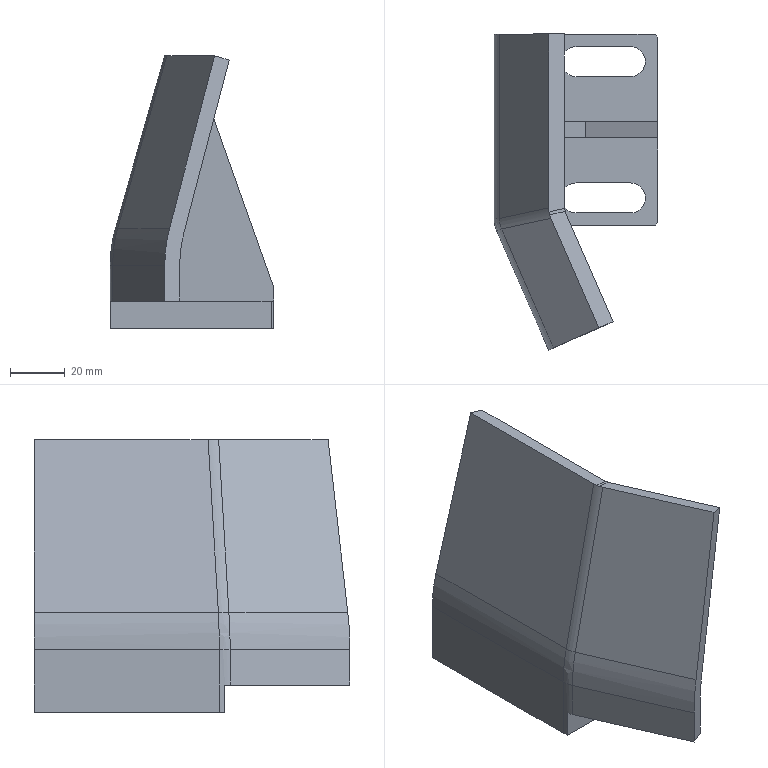Part | NX | features solid 2 | 1 solid | 44 faces | box 60 x 115.826 x 100 mm | volume 115790 mm3 | plane 28 | cylinder 14 | spline 2 | commonest cylinder face diameters 20 x5 11 x4 88 x3 100 x2
STEP:
#1=CARTESIAN_POINT('',(525.835,273.087,-27.003));
#2=VERTEX_POINT('',#1);
#3=CARTESIAN_POINT('',(545.,229.174,-27.003));
#4=VERTEX_POINT('',#3);
#5=CARTESIAN_POINT('',(525.,275.,-27.003));
#6=DIRECTION('',(0.4,-0.9165,0.));
#7=VECTOR('',#6,1000.);
#8=LINE('',#5,#7);
#9=EDGE_CURVE('',#2,#4,#8,.T.);
#10=ORIENTED_EDGE('',*,*,#9,.T.);
#11=CARTESIAN_POINT('',(546.763,229.944,-13.267));
#12=VERTEX_POINT('',#11);
#13=CARTESIAN_POINT('',(590.826,249.174,-27.003));
#14=DIRECTION('',(0.4,-0.9165,0.));
#15=DIRECTION('',(0.9165,0.4,0.));
#16=AXIS2_PLACEMENT_3D('',#13,#14,#15);
#17=CIRCLE('',#16,50.);
#18=EDGE_CURVE('',#12,#4,#17,.T.);
#19=ORIENTED_EDGE('',*,*,#18,.F.);
#20=CARTESIAN_POINT('',(527.727,273.562,-13.267));
#21=VERTEX_POINT('',#20);
#22=CARTESIAN_POINT('',(526.763,275.77,-13.267));
#23=DIRECTION('',(0.4,-0.9165,0.));
#24=VECTOR('',#23,1000.);
#25=LINE('',#22,#24);
#26=EDGE_CURVE('',#21,#12,#25,.T.);
#27=ORIENTED_EDGE('',*,*,#26,.F.);
#28=CARTESIAN_POINT('',(575.,285.436,-27.003));
#29=DIRECTION('',(-0.2436,0.9699,0.));
#30=DIRECTION('',(0.9699,0.2436,0.));
#31=AXIS2_PLACEMENT_3D('',#28,#29,#30);
#32=ELLIPSE('',#31,50.692,50.);
#33=EDGE_CURVE('',#2,#21,#32,.T.);
#34=ORIENTED_EDGE('',*,*,#33,.F.);
#35=EDGE_LOOP('',(#10,#19,#27,#34));
#36=FACE_BOUND('',#35,.T.);
#37=CARTESIAN_POINT('',(570.826,295.,-27.003));
#38=DIRECTION('',(0.4,-0.9165,0.));
#39=DIRECTION('',(-0.9165,-0.4,0.));
#40=AXIS2_PLACEMENT_3D('',#37,#38,#39);
#41=CYLINDRICAL_SURFACE('',#40,50.);
#42=ADVANCED_FACE('',(#36),#41,.T.);
#43=CARTESIAN_POINT('',(555.,279.5,-40.));
#44=VERTEX_POINT('',#43);
#45=CARTESIAN_POINT('',(575.,279.5,-40.));
#46=VERTEX_POINT('',#45);
#47=CARTESIAN_POINT('',(555.,279.5,-40.));
#48=DIRECTION('',(1.,0.,0.));
#49=VECTOR('',#48,1000.);
#50=LINE('',#47,#49);
#51=EDGE_CURVE('',#44,#46,#50,.T.);
#52=ORIENTED_EDGE('',*,*,#51,.F.);
#53=CARTESIAN_POINT('',(555.,290.5,-40.));
#54=VERTEX_POINT('',#53);
#55=CARTESIAN_POINT('',(555.,285.,-40.));
#56=DIRECTION('',(0.,0.,-1.));
#57=DIRECTION('',(1.,0.,0.));
#58=AXIS2_PLACEMENT_3D('',#55,#56,#57);
#59=CIRCLE('',#58,5.5);
#60=EDGE_CURVE('',#44,#54,#59,.T.);
#61=ORIENTED_EDGE('',*,*,#60,.T.);
#62=CARTESIAN_POINT('',(575.,290.5,-40.));
#63=VERTEX_POINT('',#62);
#64=CARTESIAN_POINT('',(575.,290.5,-40.));
#65=DIRECTION('',(-1.,0.,0.));
#66=VECTOR('',#65,1000.);
#67=LINE('',#64,#66);
#68=EDGE_CURVE('',#63,#54,#67,.T.);
#69=ORIENTED_EDGE('',*,*,#68,.F.);
#70=CARTESIAN_POINT('',(575.,285.,-40.));
#71=DIRECTION('',(0.,0.,-1.));
#72=DIRECTION('',(1.,0.,0.));
#73=AXIS2_PLACEMENT_3D('',#70,#71,#72);
#74=CIRCLE('',#73,5.5);
#75=EDGE_CURVE('',#63,#46,#74,.T.);
#76=ORIENTED_EDGE('',*,*,#75,.T.);
#77=EDGE_LOOP('',(#52,#61,#69,#76));
#78=FACE_BOUND('',#77,.T.);
#79=CARTESIAN_POINT('',(575.,340.5,-40.));
#80=VERTEX_POINT('',#79);
#81=CARTESIAN_POINT('',(555.,340.5,-40.));
#82=VERTEX_POINT('',#81);
#83=CARTESIAN_POINT('',(575.,340.5,-40.));
#84=DIRECTION('',(-1.,0.,0.));
#85=VECTOR('',#84,1000.);
#86=LINE('',#83,#85);
#87=EDGE_CURVE('',#80,#82,#86,.T.);
#88=ORIENTED_EDGE('',*,*,#87,.F.);
#89=CARTESIAN_POINT('',(575.,329.5,-40.));
#90=VERTEX_POINT('',#89);
#91=CARTESIAN_POINT('',(575.,335.,-40.));
#92=DIRECTION('',(0.,0.,-1.));
#93=DIRECTION('',(1.,0.,0.));
#94=AXIS2_PLACEMENT_3D('',#91,#92,#93);
#95=CIRCLE('',#94,5.5);
#96=EDGE_CURVE('',#80,#90,#95,.T.);
#97=ORIENTED_EDGE('',*,*,#96,.T.);
#98=CARTESIAN_POINT('',(555.,329.5,-40.));
#99=VERTEX_POINT('',#98);
#100=CARTESIAN_POINT('',(555.,329.5,-40.));
#101=DIRECTION('',(1.,0.,0.));
#102=VECTOR('',#101,1000.);
#103=LINE('',#100,#102);
#104=EDGE_CURVE('',#99,#90,#103,.T.);
#105=ORIENTED_EDGE('',*,*,#104,.F.);
#106=CARTESIAN_POINT('',(555.,335.,-40.));
#107=DIRECTION('',(0.,0.,-1.));
#108=DIRECTION('',(1.,0.,0.));
#109=AXIS2_PLACEMENT_3D('',#106,#107,#108);
#110=CIRCLE('',#109,5.5);
#111=EDGE_CURVE('',#99,#82,#110,.T.);
#112=ORIENTED_EDGE('',*,*,#111,.T.);
#113=EDGE_LOOP('',(#88,#97,#105,#112));
#114=FACE_BOUND('',#113,.T.);
#115=CARTESIAN_POINT('',(531.574,275.,-40.));
#116=VERTEX_POINT('',#115);
#117=CARTESIAN_POINT('',(584.,275.,-40.));
#118=VERTEX_POINT('',#117);
#119=CARTESIAN_POINT('',(525.,275.,-40.));
#120=DIRECTION('',(1.,0.,0.));
#121=VECTOR('',#120,1000.);
#122=LINE('',#119,#121);
#123=EDGE_CURVE('',#116,#118,#122,.T.);
#124=ORIENTED_EDGE('',*,*,#123,.T.);
#125=CARTESIAN_POINT('',(585.,276.,-40.));
#126=VERTEX_POINT('',#125);
#127=CARTESIAN_POINT('',(584.,275.,-40.));
#128=DIRECTION('',(0.7071,0.7071,0.));
#129=VECTOR('',#128,1000.);
#130=LINE('',#127,#129);
#131=EDGE_CURVE('',#118,#126,#130,.T.);
#132=ORIENTED_EDGE('',*,*,#131,.T.);
#133=CARTESIAN_POINT('',(585.,307.,-40.));
#134=VERTEX_POINT('',#133);
#135=CARTESIAN_POINT('',(585.,276.,-40.));
#136=DIRECTION('',(0.,1.,0.));
#137=VECTOR('',#136,1000.);
#138=LINE('',#135,#137);
#139=EDGE_CURVE('',#126,#134,#138,.T.);
#140=ORIENTED_EDGE('',*,*,#139,.T.);
#141=CARTESIAN_POINT('',(541.,307.,-40.));
#142=VERTEX_POINT('',#141);
#143=CARTESIAN_POINT('',(585.,307.,-40.));
#144=DIRECTION('',(-1.,0.,0.));
#145=VECTOR('',#144,1000.);
#146=LINE('',#143,#145);
#147=EDGE_CURVE('',#134,#142,#146,.T.);
#148=ORIENTED_EDGE('',*,*,#147,.T.);
#149=CARTESIAN_POINT('',(541.,313.,-40.));
#150=VERTEX_POINT('',#149);
#151=CARTESIAN_POINT('',(541.,307.,-40.));
#152=DIRECTION('',(0.,1.,0.));
#153=VECTOR('',#152,1000.);
#154=LINE('',#151,#153);
#155=EDGE_CURVE('',#142,#150,#154,.T.);
#156=ORIENTED_EDGE('',*,*,#155,.T.);
#157=CARTESIAN_POINT('',(585.,313.,-40.));
#158=VERTEX_POINT('',#157);
#159=CARTESIAN_POINT('',(585.,313.,-40.));
#160=DIRECTION('',(-1.,0.,0.));
#161=VECTOR('',#160,1000.);
#162=LINE('',#159,#161);
#163=EDGE_CURVE('',#158,#150,#162,.T.);
#164=ORIENTED_EDGE('',*,*,#163,.F.);
#165=CARTESIAN_POINT('',(585.,344.,-40.));
#166=VERTEX_POINT('',#165);
#167=CARTESIAN_POINT('',(585.,276.,-40.));
#168=DIRECTION('',(0.,1.,0.));
#169=VECTOR('',#168,1000.);
#170=LINE('',#167,#169);
#171=EDGE_CURVE('',#158,#166,#170,.T.);
#172=ORIENTED_EDGE('',*,*,#171,.T.);
#173=CARTESIAN_POINT('',(584.,345.,-40.));
#174=VERTEX_POINT('',#173);
#175=CARTESIAN_POINT('',(585.,344.,-40.));
#176=DIRECTION('',(-0.7071,0.7071,0.));
#177=VECTOR('',#176,1000.);
#178=LINE('',#175,#177);
#179=EDGE_CURVE('',#166,#174,#178,.T.);
#180=ORIENTED_EDGE('',*,*,#179,.T.);
#181=CARTESIAN_POINT('',(531.,345.,-40.));
#182=VERTEX_POINT('',#181);
#183=CARTESIAN_POINT('',(584.,345.,-40.));
#184=DIRECTION('',(-1.,0.,0.));
#185=VECTOR('',#184,1000.);
#186=LINE('',#183,#185);
#187=EDGE_CURVE('',#174,#182,#186,.T.);
#188=ORIENTED_EDGE('',*,*,#187,.T.);
#189=CARTESIAN_POINT('',(531.,278.339,-40.));
#190=VERTEX_POINT('',#189);
#191=CARTESIAN_POINT('',(531.,275.,-40.));
#192=DIRECTION('',(0.,1.,0.));
#193=VECTOR('',#192,1000.);
#194=LINE('',#191,#193);
#195=EDGE_CURVE('',#190,#182,#194,.T.);
#196=ORIENTED_EDGE('',*,*,#195,.F.);
#197=CARTESIAN_POINT('',(541.,278.339,-40.));
#198=DIRECTION('',(0.,0.,1.));
#199=DIRECTION('',(-1.,0.,0.));
#200=AXIS2_PLACEMENT_3D('',#197,#198,#199);
#201=CIRCLE('',#200,10.);
#202=EDGE_CURVE('',#116,#190,#201,.F.);
#203=ORIENTED_EDGE('',*,*,#202,.F.);
#204=EDGE_LOOP('',(#124,#132,#140,#148,#156,#164,#172,#180,#188,#196,#203));
#205=FACE_BOUND('',#204,.T.);
#206=CARTESIAN_POINT('',(525.,275.,-40.));
#207=DIRECTION('',(0.,0.,-1.));
#208=DIRECTION('',(-1.,0.,0.));
#209=AXIS2_PLACEMENT_3D('',#206,#207,#208);
#210=PLANE('',#209);
#211=ADVANCED_FACE('',(#78,#114,#205),#210,.F.);
#212=CARTESIAN_POINT('',(525.,277.087,-27.003));
#213=VERTEX_POINT('',#212);
#214=CARTESIAN_POINT('',(525.,345.,-27.003));
#215=VERTEX_POINT('',#214);
#216=CARTESIAN_POINT('',(525.,275.,-27.003));
#217=DIRECTION('',(0.,1.,0.));
#218=VECTOR('',#217,1000.);
#219=LINE('',#216,#218);
#220=EDGE_CURVE('',#213,#215,#219,.T.);
#221=ORIENTED_EDGE('',*,*,#220,.T.);
#222=CARTESIAN_POINT('',(525.,345.,-50.));
#223=VERTEX_POINT('',#222);
#224=CARTESIAN_POINT('',(525.,345.,-40.));
#225=DIRECTION('',(0.,0.,-1.));
#226=VECTOR('',#225,1000.);
#227=LINE('',#224,#226);
#228=EDGE_CURVE('',#215,#223,#227,.T.);
#229=ORIENTED_EDGE('',*,*,#228,.T.);
#230=CARTESIAN_POINT('',(525.,277.087,-50.));
#231=VERTEX_POINT('',#230);
#232=CARTESIAN_POINT('',(525.,345.,-50.));
#233=DIRECTION('',(0.,-1.,0.));
#234=VECTOR('',#233,1000.);
#235=LINE('',#232,#234);
#236=EDGE_CURVE('',#223,#231,#235,.T.);
#237=ORIENTED_EDGE('',*,*,#236,.T.);
#238=CARTESIAN_POINT('',(525.,277.087,-40.));
#239=DIRECTION('',(0.,0.,-1.));
#240=VECTOR('',#239,1000.);
#241=LINE('',#238,#240);
#242=EDGE_CURVE('',#213,#231,#241,.T.);
#243=ORIENTED_EDGE('',*,*,#242,.F.);
#244=EDGE_LOOP('',(#221,#229,#237,#243));
#245=FACE_BOUND('',#244,.T.);
#246=CARTESIAN_POINT('',(525.,345.,-40.));
#247=DIRECTION('',(-1.,0.,0.));
#248=DIRECTION('',(0.,0.,1.));
#249=AXIS2_PLACEMENT_3D('',#246,#247,#248);
#250=PLANE('',#249);
#251=ADVANCED_FACE('',(#245),#250,.T.);
#252=CARTESIAN_POINT('',(525.22,275.,-50.));
#253=VERTEX_POINT('',#252);
#254=CARTESIAN_POINT('',(584.,275.,-50.));
#255=VERTEX_POINT('',#254);
#256=CARTESIAN_POINT('',(525.,275.,-50.));
#257=DIRECTION('',(1.,0.,0.));
#258=VECTOR('',#257,1000.);
#259=LINE('',#256,#258);
#260=EDGE_CURVE('',#253,#255,#259,.T.);
#261=ORIENTED_EDGE('',*,*,#260,.T.);
#262=CARTESIAN_POINT('',(584.,275.,-40.));
#263=DIRECTION('',(0.,0.,-1.));
#264=VECTOR('',#263,1000.);
#265=LINE('',#262,#264);
#266=EDGE_CURVE('',#118,#255,#265,.T.);
#267=ORIENTED_EDGE('',*,*,#266,.F.);
#268=ORIENTED_EDGE('',*,*,#123,.F.);
#269=CARTESIAN_POINT('',(525.22,275.,-40.));
#270=VERTEX_POINT('',#269);
#271=CARTESIAN_POINT('',(525.,275.,-40.));
#272=DIRECTION('',(1.,0.,0.));
#273=VECTOR('',#272,1000.);
#274=LINE('',#271,#273);
#275=EDGE_CURVE('',#270,#116,#274,.T.);
#276=ORIENTED_EDGE('',*,*,#275,.F.);
#277=CARTESIAN_POINT('',(525.22,275.,-50.));
#278=DIRECTION('',(0.,0.,-1.));
#279=VECTOR('',#278,1000.);
#280=LINE('',#277,#279);
#281=EDGE_CURVE('',#253,#270,#280,.F.);
#282=ORIENTED_EDGE('',*,*,#281,.F.);
#283=EDGE_LOOP('',(#261,#267,#268,#276,#282));
#284=FACE_BOUND('',#283,.T.);
#285=CARTESIAN_POINT('',(525.,275.,-40.));
#286=DIRECTION('',(0.,-1.,0.));
#287=DIRECTION('',(0.,0.,1.));
#288=AXIS2_PLACEMENT_3D('',#285,#286,#287);
#289=PLANE('',#288);
#290=ADVANCED_FACE('',(#284),#289,.T.);
#291=CARTESIAN_POINT('',(585.,276.,-50.));
#292=VERTEX_POINT('',#291);
#293=CARTESIAN_POINT('',(584.,275.,-50.));
#294=DIRECTION('',(0.7071,0.7071,0.));
#295=VECTOR('',#294,1000.);
#296=LINE('',#293,#295);
#297=EDGE_CURVE('',#255,#292,#296,.T.);
#298=ORIENTED_EDGE('',*,*,#297,.T.);
#299=CARTESIAN_POINT('',(585.,276.,-40.));
#300=DIRECTION('',(0.,0.,-1.));
#301=VECTOR('',#300,1000.);
#302=LINE('',#299,#301);
#303=EDGE_CURVE('',#126,#292,#302,.T.);
#304=ORIENTED_EDGE('',*,*,#303,.F.);
#305=ORIENTED_EDGE('',*,*,#131,.F.);
#306=ORIENTED_EDGE('',*,*,#266,.T.);
#307=EDGE_LOOP('',(#298,#304,#305,#306));
#308=FACE_BOUND('',#307,.T.);
#309=CARTESIAN_POINT('',(584.,275.,-40.));
#310=DIRECTION('',(0.7071,-0.7071,0.));
#311=DIRECTION('',(-0.7071,-0.7071,0.));
#312=AXIS2_PLACEMENT_3D('',#309,#310,#311);
#313=PLANE('',#312);
#314=ADVANCED_FACE('',(#308),#313,.T.);
#315=CARTESIAN_POINT('',(585.,344.,-50.));
#316=VERTEX_POINT('',#315);
#317=CARTESIAN_POINT('',(585.,276.,-50.));
#318=DIRECTION('',(0.,1.,0.));
#319=VECTOR('',#318,1000.);
#320=LINE('',#317,#319);
#321=EDGE_CURVE('',#292,#316,#320,.T.);
#322=ORIENTED_EDGE('',*,*,#321,.T.);
#323=CARTESIAN_POINT('',(585.,344.,-40.));
#324=DIRECTION('',(0.,0.,-1.));
#325=VECTOR('',#324,1000.);
#326=LINE('',#323,#325);
#327=EDGE_CURVE('',#166,#316,#326,.T.);
#328=ORIENTED_EDGE('',*,*,#327,.F.);
#329=ORIENTED_EDGE('',*,*,#171,.F.);
#330=CARTESIAN_POINT('',(585.,313.,-35.));
#331=VERTEX_POINT('',#330);
#332=CARTESIAN_POINT('',(585.,313.,-35.));
#333=DIRECTION('',(0.,0.,-1.));
#334=VECTOR('',#333,1000.);
#335=LINE('',#332,#334);
#336=EDGE_CURVE('',#331,#158,#335,.T.);
#337=ORIENTED_EDGE('',*,*,#336,.F.);
#338=CARTESIAN_POINT('',(585.,307.,-35.));
#339=VERTEX_POINT('',#338);
#340=CARTESIAN_POINT('',(585.,307.,-35.));
#341=DIRECTION('',(0.,1.,0.));
#342=VECTOR('',#341,1000.);
#343=LINE('',#340,#342);
#344=EDGE_CURVE('',#339,#331,#343,.T.);
#345=ORIENTED_EDGE('',*,*,#344,.F.);
#346=CARTESIAN_POINT('',(585.,307.,-35.));
#347=DIRECTION('',(0.,0.,-1.));
#348=VECTOR('',#347,1000.);
#349=LINE('',#346,#348);
#350=EDGE_CURVE('',#339,#134,#349,.T.);
#351=ORIENTED_EDGE('',*,*,#350,.T.);
#352=ORIENTED_EDGE('',*,*,#139,.F.);
#353=ORIENTED_EDGE('',*,*,#303,.T.);
#354=EDGE_LOOP('',(#322,#328,#329,#337,#345,#351,#352,#353));
#355=FACE_BOUND('',#354,.T.);
#356=CARTESIAN_POINT('',(585.,276.,-40.));
#357=DIRECTION('',(1.,0.,0.));
#358=DIRECTION('',(0.,-1.,0.));
#359=AXIS2_PLACEMENT_3D('',#356,#357,#358);
#360=PLANE('',#359);
#361=ADVANCED_FACE('',(#355),#360,.T.);
#362=CARTESIAN_POINT('',(584.,345.,-50.));
#363=VERTEX_POINT('',#362);
#364=CARTESIAN_POINT('',(585.,344.,-50.));
#365=DIRECTION('',(-0.7071,0.7071,0.));
#366=VECTOR('',#365,1000.);
#367=LINE('',#364,#366);
#368=EDGE_CURVE('',#316,#363,#367,.T.);
#369=ORIENTED_EDGE('',*,*,#368,.T.);
#370=CARTESIAN_POINT('',(584.,345.,-40.));
#371=DIRECTION('',(0.,0.,-1.));
#372=VECTOR('',#371,1000.);
#373=LINE('',#370,#372);
#374=EDGE_CURVE('',#174,#363,#373,.T.);
#375=ORIENTED_EDGE('',*,*,#374,.F.);
#376=ORIENTED_EDGE('',*,*,#179,.F.);
#377=ORIENTED_EDGE('',*,*,#327,.T.);
#378=EDGE_LOOP('',(#369,#375,#376,#377));
#379=FACE_BOUND('',#378,.T.);
#380=CARTESIAN_POINT('',(585.,344.,-40.));
#381=DIRECTION('',(0.7071,0.7071,0.));
#382=DIRECTION('',(0.7071,-0.7071,0.));
#383=AXIS2_PLACEMENT_3D('',#380,#381,#382);
#384=PLANE('',#383);
#385=ADVANCED_FACE('',(#379),#384,.T.);
#386=CARTESIAN_POINT('',(555.,279.5,-50.));
#387=VERTEX_POINT('',#386);
#388=CARTESIAN_POINT('',(575.,279.5,-50.));
#389=VERTEX_POINT('',#388);
#390=CARTESIAN_POINT('',(555.,279.5,-50.));
#391=DIRECTION('',(1.,0.,0.));
#392=VECTOR('',#391,1000.);
#393=LINE('',#390,#392);
#394=EDGE_CURVE('',#387,#389,#393,.T.);
#395=ORIENTED_EDGE('',*,*,#394,.F.);
#396=CARTESIAN_POINT('',(555.,279.5,-40.));
#397=DIRECTION('',(0.,0.,-1.));
#398=VECTOR('',#397,1000.);
#399=LINE('',#396,#398);
#400=EDGE_CURVE('',#44,#387,#399,.T.);
#401=ORIENTED_EDGE('',*,*,#400,.F.);
#402=ORIENTED_EDGE('',*,*,#51,.T.);
#403=CARTESIAN_POINT('',(575.,279.5,-40.));
#404=DIRECTION('',(0.,0.,-1.));
#405=VECTOR('',#404,1000.);
#406=LINE('',#403,#405);
#407=EDGE_CURVE('',#46,#389,#406,.T.);
#408=ORIENTED_EDGE('',*,*,#407,.T.);
#409=EDGE_LOOP('',(#395,#401,#402,#408));
#410=FACE_BOUND('',#409,.T.);
#411=CARTESIAN_POINT('',(555.,279.5,-40.));
#412=DIRECTION('',(0.,-1.,0.));
#413=DIRECTION('',(0.,0.,1.));
#414=AXIS2_PLACEMENT_3D('',#411,#412,#413);
#415=PLANE('',#414);
#416=ADVANCED_FACE('',(#410),#415,.F.);
#417=CARTESIAN_POINT('',(555.,290.5,-50.));
#418=VERTEX_POINT('',#417);
#419=CARTESIAN_POINT('',(555.,285.,-50.));
#420=DIRECTION('',(0.,0.,-1.));
#421=DIRECTION('',(1.,0.,0.));
#422=AXIS2_PLACEMENT_3D('',#419,#420,#421);
#423=CIRCLE('',#422,5.5);
#424=EDGE_CURVE('',#387,#418,#423,.T.);
#425=ORIENTED_EDGE('',*,*,#424,.T.);
#426=CARTESIAN_POINT('',(555.,290.5,-40.));
#427=DIRECTION('',(0.,0.,-1.));
#428=VECTOR('',#427,1000.);
#429=LINE('',#426,#428);
#430=EDGE_CURVE('',#54,#418,#429,.T.);
#431=ORIENTED_EDGE('',*,*,#430,.F.);
#432=ORIENTED_EDGE('',*,*,#60,.F.);
#433=ORIENTED_EDGE('',*,*,#400,.T.);
#434=EDGE_LOOP('',(#425,#431,#432,#433));
#435=FACE_BOUND('',#434,.T.);
#436=CARTESIAN_POINT('',(555.,285.,-40.));
#437=DIRECTION('',(0.,0.,-1.));
#438=DIRECTION('',(-1.,0.,0.));
#439=AXIS2_PLACEMENT_3D('',#436,#437,#438);
#440=CYLINDRICAL_SURFACE('',#439,5.5);
#441=ADVANCED_FACE('',(#435),#440,.F.);
#442=CARTESIAN_POINT('',(575.,290.5,-50.));
#443=VERTEX_POINT('',#442);
#444=CARTESIAN_POINT('',(575.,290.5,-50.));
#445=DIRECTION('',(-1.,0.,0.));
#446=VECTOR('',#445,1000.);
#447=LINE('',#444,#446);
#448=EDGE_CURVE('',#443,#418,#447,.T.);
#449=ORIENTED_EDGE('',*,*,#448,.F.);
#450=CARTESIAN_POINT('',(575.,290.5,-40.));
#451=DIRECTION('',(0.,0.,-1.));
#452=VECTOR('',#451,1000.);
#453=LINE('',#450,#452);
#454=EDGE_CURVE('',#63,#443,#453,.T.);
#455=ORIENTED_EDGE('',*,*,#454,.F.);
#456=ORIENTED_EDGE('',*,*,#68,.T.);
#457=ORIENTED_EDGE('',*,*,#430,.T.);
#458=EDGE_LOOP('',(#449,#455,#456,#457));
#459=FACE_BOUND('',#458,.T.);
#460=CARTESIAN_POINT('',(575.,290.5,-40.));
#461=DIRECTION('',(0.,1.,0.));
#462=DIRECTION('',(0.,0.,-1.));
#463=AXIS2_PLACEMENT_3D('',#460,#461,#462);
#464=PLANE('',#463);
#465=ADVANCED_FACE('',(#459),#464,.F.);
#466=CARTESIAN_POINT('',(575.,340.5,-50.));
#467=VERTEX_POINT('',#466);
#468=CARTESIAN_POINT('',(555.,340.5,-50.));
#469=VERTEX_POINT('',#468);
#470=CARTESIAN_POINT('',(575.,340.5,-50.));
#471=DIRECTION('',(-1.,0.,0.));
#472=VECTOR('',#471,1000.);
#473=LINE('',#470,#472);
#474=EDGE_CURVE('',#467,#469,#473,.T.);
#475=ORIENTED_EDGE('',*,*,#474,.F.);
#476=CARTESIAN_POINT('',(575.,340.5,-40.));
#477=DIRECTION('',(0.,0.,-1.));
#478=VECTOR('',#477,1000.);
#479=LINE('',#476,#478);
#480=EDGE_CURVE('',#80,#467,#479,.T.);
#481=ORIENTED_EDGE('',*,*,#480,.F.);
#482=ORIENTED_EDGE('',*,*,#87,.T.);
#483=CARTESIAN_POINT('',(555.,340.5,-40.));
#484=DIRECTION('',(0.,0.,-1.));
#485=VECTOR('',#484,1000.);
#486=LINE('',#483,#485);
#487=EDGE_CURVE('',#82,#469,#486,.T.);
#488=ORIENTED_EDGE('',*,*,#487,.T.);
#489=EDGE_LOOP('',(#475,#481,#482,#488));
#490=FACE_BOUND('',#489,.T.);
#491=CARTESIAN_POINT('',(575.,340.5,-40.));
#492=DIRECTION('',(0.,1.,0.));
#493=DIRECTION('',(0.,0.,-1.));
#494=AXIS2_PLACEMENT_3D('',#491,#492,#493);
#495=PLANE('',#494);
#496=ADVANCED_FACE('',(#490),#495,.F.);
#497=CARTESIAN_POINT('',(575.,329.5,-50.));
#498=VERTEX_POINT('',#497);
#499=CARTESIAN_POINT('',(575.,335.,-50.));
#500=DIRECTION('',(0.,0.,-1.));
#501=DIRECTION('',(1.,0.,0.));
#502=AXIS2_PLACEMENT_3D('',#499,#500,#501);
#503=CIRCLE('',#502,5.5);
#504=EDGE_CURVE('',#467,#498,#503,.T.);
#505=ORIENTED_EDGE('',*,*,#504,.T.);
#506=CARTESIAN_POINT('',(575.,329.5,-40.));
#507=DIRECTION('',(0.,0.,-1.));
#508=VECTOR('',#507,1000.);
#509=LINE('',#506,#508);
#510=EDGE_CURVE('',#90,#498,#509,.T.);
#511=ORIENTED_EDGE('',*,*,#510,.F.);
#512=ORIENTED_EDGE('',*,*,#96,.F.);
#513=ORIENTED_EDGE('',*,*,#480,.T.);
#514=EDGE_LOOP('',(#505,#511,#512,#513));
#515=FACE_BOUND('',#514,.T.);
#516=CARTESIAN_POINT('',(575.,335.,-40.));
#517=DIRECTION('',(0.,0.,-1.));
#518=DIRECTION('',(-1.,0.,0.));
#519=AXIS2_PLACEMENT_3D('',#516,#517,#518);
#520=CYLINDRICAL_SURFACE('',#519,5.5);
#521=ADVANCED_FACE('',(#515),#520,.F.);
#522=CARTESIAN_POINT('',(555.,329.5,-50.));
#523=VERTEX_POINT('',#522);
#524=CARTESIAN_POINT('',(555.,329.5,-50.));
#525=DIRECTION('',(1.,0.,0.));
#526=VECTOR('',#525,1000.);
#527=LINE('',#524,#526);
#528=EDGE_CURVE('',#523,#498,#527,.T.);
#529=ORIENTED_EDGE('',*,*,#528,.F.);
#530=CARTESIAN_POINT('',(555.,329.5,-40.));
#531=DIRECTION('',(0.,0.,-1.));
#532=VECTOR('',#531,1000.);
#533=LINE('',#530,#532);
#534=EDGE_CURVE('',#99,#523,#533,.T.);
#535=ORIENTED_EDGE('',*,*,#534,.F.);
#536=ORIENTED_EDGE('',*,*,#104,.T.);
#537=ORIENTED_EDGE('',*,*,#510,.T.);
#538=EDGE_LOOP('',(#529,#535,#536,#537));
#539=FACE_BOUND('',#538,.T.);
#540=CARTESIAN_POINT('',(555.,329.5,-40.));
#541=DIRECTION('',(0.,-1.,0.));
#542=DIRECTION('',(0.,0.,1.));
#543=AXIS2_PLACEMENT_3D('',#540,#541,#542);
#544=PLANE('',#543);
#545=ADVANCED_FACE('',(#539),#544,.F.);
#546=CARTESIAN_POINT('',(575.,285.,-50.));
#547=DIRECTION('',(0.,0.,-1.));
#548=DIRECTION('',(1.,0.,0.));
#549=AXIS2_PLACEMENT_3D('',#546,#547,#548);
#550=CIRCLE('',#549,5.5);
#551=EDGE_CURVE('',#443,#389,#550,.T.);
#552=ORIENTED_EDGE('',*,*,#551,.T.);
#553=ORIENTED_EDGE('',*,*,#407,.F.);
#554=ORIENTED_EDGE('',*,*,#75,.F.);
#555=ORIENTED_EDGE('',*,*,#454,.T.);
#556=EDGE_LOOP('',(#552,#553,#554,#555));
#557=FACE_BOUND('',#556,.T.);
#558=CARTESIAN_POINT('',(575.,285.,-40.));
#559=DIRECTION('',(0.,0.,-1.));
#560=DIRECTION('',(-1.,0.,0.));
#561=AXIS2_PLACEMENT_3D('',#558,#559,#560);
#562=CYLINDRICAL_SURFACE('',#561,5.5);
#563=ADVANCED_FACE('',(#557),#562,.F.);
#564=CARTESIAN_POINT('',(555.,335.,-50.));
#565=DIRECTION('',(0.,0.,-1.));
#566=DIRECTION('',(1.,0.,0.));
#567=AXIS2_PLACEMENT_3D('',#564,#565,#566);
#568=CIRCLE('',#567,5.5);
#569=EDGE_CURVE('',#523,#469,#568,.T.);
#570=ORIENTED_EDGE('',*,*,#569,.T.);
#571=ORIENTED_EDGE('',*,*,#487,.F.);
#572=ORIENTED_EDGE('',*,*,#111,.F.);
#573=ORIENTED_EDGE('',*,*,#534,.T.);
#574=EDGE_LOOP('',(#570,#571,#572,#573));
#575=FACE_BOUND('',#574,.T.);
#576=CARTESIAN_POINT('',(555.,335.,-40.));
#577=DIRECTION('',(0.,0.,-1.));
#578=DIRECTION('',(-1.,0.,0.));
#579=AXIS2_PLACEMENT_3D('',#576,#577,#578);
#580=CYLINDRICAL_SURFACE('',#579,5.5);
#581=ADVANCED_FACE('',(#575),#580,.F.);
#582=CARTESIAN_POINT('',(584.,345.,-50.));
#583=DIRECTION('',(-1.,0.,0.));
#584=VECTOR('',#583,1000.);
#585=LINE('',#582,#584);
#586=EDGE_CURVE('',#363,#223,#585,.T.);
#587=ORIENTED_EDGE('',*,*,#586,.T.);
#588=ORIENTED_EDGE('',*,*,#228,.F.);
#589=CARTESIAN_POINT('',(526.924,345.,-13.267));
#590=VERTEX_POINT('',#589);
#591=CARTESIAN_POINT('',(575.,345.,-27.003));
#592=DIRECTION('',(0.,-1.,0.));
#593=DIRECTION('',(1.,0.,0.));
#594=AXIS2_PLACEMENT_3D('',#591,#592,#593);
#595=CIRCLE('',#594,50.);
#596=EDGE_CURVE('',#590,#215,#595,.T.);
#597=ORIENTED_EDGE('',*,*,#596,.F.);
#598=CARTESIAN_POINT('',(545.,345.,50.));
#599=VERTEX_POINT('',#598);
#600=CARTESIAN_POINT('',(526.924,345.,-13.267));
#601=DIRECTION('',(0.2747,0.,0.9615));
#602=VECTOR('',#601,1000.);
#603=LINE('',#600,#602);
#604=EDGE_CURVE('',#590,#599,#603,.T.);
#605=ORIENTED_EDGE('',*,*,#604,.T.);
#606=CARTESIAN_POINT('',(550.769,345.,48.352));
#607=VERTEX_POINT('',#606);
#608=CARTESIAN_POINT('',(545.,345.,50.));
#609=DIRECTION('',(0.9615,0.,-0.2747));
#610=VECTOR('',#609,1000.);
#611=LINE('',#608,#610);
#612=EDGE_CURVE('',#599,#607,#611,.T.);
#613=ORIENTED_EDGE('',*,*,#612,.T.);
#614=CARTESIAN_POINT('',(532.693,345.,-14.915));
#615=VERTEX_POINT('',#614);
#616=CARTESIAN_POINT('',(532.693,345.,-14.915));
#617=DIRECTION('',(0.2747,0.,0.9615));
#618=VECTOR('',#617,1000.);
#619=LINE('',#616,#618);
#620=EDGE_CURVE('',#615,#607,#619,.T.);
#621=ORIENTED_EDGE('',*,*,#620,.F.);
#622=CARTESIAN_POINT('',(531.,345.,-27.003));
#623=VERTEX_POINT('',#622);
#624=CARTESIAN_POINT('',(575.,345.,-27.003));
#625=DIRECTION('',(0.,-1.,0.));
#626=DIRECTION('',(1.,0.,0.));
#627=AXIS2_PLACEMENT_3D('',#624,#625,#626);
#628=CIRCLE('',#627,44.);
#629=EDGE_CURVE('',#615,#623,#628,.T.);
#630=ORIENTED_EDGE('',*,*,#629,.T.);
#631=CARTESIAN_POINT('',(531.,345.,-27.003));
#632=DIRECTION('',(0.,0.,-1.));
#633=VECTOR('',#632,1000.);
#634=LINE('',#631,#633);
#635=EDGE_CURVE('',#623,#182,#634,.T.);
#636=ORIENTED_EDGE('',*,*,#635,.T.);
#637=ORIENTED_EDGE('',*,*,#187,.F.);
#638=ORIENTED_EDGE('',*,*,#374,.T.);
#639=EDGE_LOOP('',(#587,#588,#597,#605,#613,#621,#630,#636,#637,#638));
#640=FACE_BOUND('',#639,.T.);
#641=CARTESIAN_POINT('',(584.,345.,-40.));
#642=DIRECTION('',(0.,1.,0.));
#643=DIRECTION('',(1.,0.,0.));
#644=AXIS2_PLACEMENT_3D('',#641,#642,#643);
#645=PLANE('',#644);
#646=ADVANCED_FACE('',(#640),#645,.T.);
#647=ORIENTED_EDGE('',*,*,#474,.T.);
#648=ORIENTED_EDGE('',*,*,#569,.F.);
#649=ORIENTED_EDGE('',*,*,#528,.T.);
#650=ORIENTED_EDGE('',*,*,#504,.F.);
#651=EDGE_LOOP('',(#647,#648,#649,#650));
#652=FACE_BOUND('',#651,.T.);
#653=ORIENTED_EDGE('',*,*,#394,.T.);
#654=ORIENTED_EDGE('',*,*,#551,.F.);
#655=ORIENTED_EDGE('',*,*,#448,.T.);
#656=ORIENTED_EDGE('',*,*,#424,.F.);
#657=EDGE_LOOP('',(#653,#654,#655,#656));
#658=FACE_BOUND('',#657,.T.);
#659=ORIENTED_EDGE('',*,*,#236,.F.);
#660=ORIENTED_EDGE('',*,*,#586,.F.);
#661=ORIENTED_EDGE('',*,*,#368,.F.);
#662=ORIENTED_EDGE('',*,*,#321,.F.);
#663=ORIENTED_EDGE('',*,*,#297,.F.);
#664=ORIENTED_EDGE('',*,*,#260,.F.);
#665=CARTESIAN_POINT('',(535.,277.087,-50.));
#666=DIRECTION('',(0.,0.,1.));
#667=DIRECTION('',(-1.,0.,0.));
#668=AXIS2_PLACEMENT_3D('',#665,#666,#667);
#669=CIRCLE('',#668,10.);
#670=EDGE_CURVE('',#231,#253,#669,.T.);
#671=ORIENTED_EDGE('',*,*,#670,.F.);
#672=EDGE_LOOP('',(#659,#660,#661,#662,#663,#664,#671));
#673=FACE_BOUND('',#672,.T.);
#674=CARTESIAN_POINT('',(525.,275.,-50.));
#675=DIRECTION('',(0.,0.,-1.));
#676=DIRECTION('',(-1.,0.,0.));
#677=AXIS2_PLACEMENT_3D('',#674,#675,#676);
#678=PLANE('',#677);
#679=ADVANCED_FACE('',(#652,#658,#673),#678,.T.);
#680=CARTESIAN_POINT('',(548.383,313.,40.));
#681=VERTEX_POINT('',#680);
#682=CARTESIAN_POINT('',(558.383,313.,40.));
#683=VERTEX_POINT('',#682);
#684=CARTESIAN_POINT('',(548.383,313.,40.));
#685=DIRECTION('',(1.,0.,0.));
#686=VECTOR('',#685,1000.);
#687=LINE('',#684,#686);
#688=EDGE_CURVE('',#681,#683,#687,.T.);
#689=ORIENTED_EDGE('',*,*,#688,.F.);
#690=CARTESIAN_POINT('',(548.383,307.,40.));
#691=VERTEX_POINT('',#690);
#692=CARTESIAN_POINT('',(548.383,307.,40.));
#693=DIRECTION('',(0.,1.,0.));
#694=VECTOR('',#693,1000.);
#695=LINE('',#692,#694);
#696=EDGE_CURVE('',#691,#681,#695,.T.);
#697=ORIENTED_EDGE('',*,*,#696,.F.);
#698=CARTESIAN_POINT('',(558.383,307.,40.));
#699=VERTEX_POINT('',#698);
#700=CARTESIAN_POINT('',(548.383,307.,40.));
#701=DIRECTION('',(1.,0.,0.));
#702=VECTOR('',#701,1000.);
#703=LINE('',#700,#702);
#704=EDGE_CURVE('',#691,#699,#703,.T.);
#705=ORIENTED_EDGE('',*,*,#704,.T.);
#706=CARTESIAN_POINT('',(558.383,307.,40.));
#707=DIRECTION('',(0.,1.,0.));
#708=VECTOR('',#707,1000.);
#709=LINE('',#706,#708);
#710=EDGE_CURVE('',#699,#683,#709,.T.);
#711=ORIENTED_EDGE('',*,*,#710,.T.);
#712=EDGE_LOOP('',(#689,#697,#705,#711));
#713=FACE_BOUND('',#712,.T.);
#714=CARTESIAN_POINT('',(548.383,307.,40.));
#715=DIRECTION('',(0.,0.,-1.));
#716=DIRECTION('',(-1.,0.,0.));
#717=AXIS2_PLACEMENT_3D('',#714,#715,#716);
#718=PLANE('',#717);
#719=ADVANCED_FACE('',(#713),#718,.F.);
#720=CARTESIAN_POINT('',(558.383,313.,40.));
#721=DIRECTION('',(0.3345,0.,-0.9424));
#722=VECTOR('',#721,1000.);
#723=LINE('',#720,#722);
#724=EDGE_CURVE('',#683,#331,#723,.T.);
#725=ORIENTED_EDGE('',*,*,#724,.F.);
#726=ORIENTED_EDGE('',*,*,#710,.F.);
#727=CARTESIAN_POINT('',(558.383,307.,40.));
#728=DIRECTION('',(0.3345,0.,-0.9424));
#729=VECTOR('',#728,1000.);
#730=LINE('',#727,#729);
#731=EDGE_CURVE('',#699,#339,#730,.T.);
#732=ORIENTED_EDGE('',*,*,#731,.T.);
#733=ORIENTED_EDGE('',*,*,#344,.T.);
#734=EDGE_LOOP('',(#725,#726,#732,#733));
#735=FACE_BOUND('',#734,.T.);
#736=CARTESIAN_POINT('',(558.383,307.,40.));
#737=DIRECTION('',(-0.9424,0.,-0.3345));
#738=DIRECTION('',(-0.3345,0.,0.9424));
#739=AXIS2_PLACEMENT_3D('',#736,#737,#738);
#740=PLANE('',#739);
#741=ADVANCED_FACE('',(#735),#740,.F.);
#742=ORIENTED_EDGE('',*,*,#147,.F.);
#743=ORIENTED_EDGE('',*,*,#350,.F.);
#744=ORIENTED_EDGE('',*,*,#731,.F.);
#745=ORIENTED_EDGE('',*,*,#704,.F.);
#746=CARTESIAN_POINT('',(532.693,307.,-14.915));
#747=VERTEX_POINT('',#746);
#748=CARTESIAN_POINT('',(532.693,307.,-14.915));
#749=DIRECTION('',(0.2747,0.,0.9615));
#750=VECTOR('',#749,1000.);
#751=LINE('',#748,#750);
#752=EDGE_CURVE('',#747,#691,#751,.T.);
#753=ORIENTED_EDGE('',*,*,#752,.F.);
#754=CARTESIAN_POINT('',(531.,307.,-27.003));
#755=VERTEX_POINT('',#754);
#756=CARTESIAN_POINT('',(575.,307.,-27.003));
#757=DIRECTION('',(0.,-1.,0.));
#758=DIRECTION('',(1.,0.,0.));
#759=AXIS2_PLACEMENT_3D('',#756,#757,#758);
#760=CIRCLE('',#759,44.);
#761=EDGE_CURVE('',#747,#755,#760,.T.);
#762=ORIENTED_EDGE('',*,*,#761,.T.);
#763=CARTESIAN_POINT('',(531.,307.,-30.));
#764=VERTEX_POINT('',#763);
#765=CARTESIAN_POINT('',(531.,307.,-27.003));
#766=DIRECTION('',(0.,0.,-1.));
#767=VECTOR('',#766,1000.);
#768=LINE('',#765,#767);
#769=EDGE_CURVE('',#755,#764,#768,.T.);
#770=ORIENTED_EDGE('',*,*,#769,.T.);
#771=CARTESIAN_POINT('',(541.,307.,-40.));
#772=DIRECTION('',(-0.7071,0.,0.7071));
#773=VECTOR('',#772,1000.);
#774=LINE('',#771,#773);
#775=EDGE_CURVE('',#142,#764,#774,.T.);
#776=ORIENTED_EDGE('',*,*,#775,.F.);
#777=EDGE_LOOP('',(#742,#743,#744,#745,#753,#762,#770,#776));
#778=FACE_BOUND('',#777,.T.);
#779=CARTESIAN_POINT('',(575.,307.,-27.003));
#780=DIRECTION('',(0.,1.,0.));
#781=DIRECTION('',(0.,0.,-1.));
#782=AXIS2_PLACEMENT_3D('',#779,#780,#781);
#783=PLANE('',#782);
#784=ADVANCED_FACE('',(#778),#783,.F.);
#785=CARTESIAN_POINT('',(531.,313.,-30.));
#786=VERTEX_POINT('',#785);
#787=CARTESIAN_POINT('',(541.,313.,-40.));
#788=DIRECTION('',(-0.7071,0.,0.7071));
#789=VECTOR('',#788,1000.);
#790=LINE('',#787,#789);
#791=EDGE_CURVE('',#150,#786,#790,.T.);
#792=ORIENTED_EDGE('',*,*,#791,.T.);
#793=CARTESIAN_POINT('',(531.,313.,-27.003));
#794=VERTEX_POINT('',#793);
#795=CARTESIAN_POINT('',(531.,313.,-27.003));
#796=DIRECTION('',(0.,0.,-1.));
#797=VECTOR('',#796,1000.);
#798=LINE('',#795,#797);
#799=EDGE_CURVE('',#794,#786,#798,.T.);
#800=ORIENTED_EDGE('',*,*,#799,.F.);
#801=CARTESIAN_POINT('',(532.693,313.,-14.915));
#802=VERTEX_POINT('',#801);
#803=CARTESIAN_POINT('',(575.,313.,-27.003));
#804=DIRECTION('',(0.,-1.,0.));
#805=DIRECTION('',(1.,0.,0.));
#806=AXIS2_PLACEMENT_3D('',#803,#804,#805);
#807=CIRCLE('',#806,44.);
#808=EDGE_CURVE('',#802,#794,#807,.T.);
#809=ORIENTED_EDGE('',*,*,#808,.F.);
#810=CARTESIAN_POINT('',(532.693,313.,-14.915));
#811=DIRECTION('',(0.2747,0.,0.9615));
#812=VECTOR('',#811,1000.);
#813=LINE('',#810,#812);
#814=EDGE_CURVE('',#802,#681,#813,.T.);
#815=ORIENTED_EDGE('',*,*,#814,.T.);
#816=ORIENTED_EDGE('',*,*,#688,.T.);
#817=ORIENTED_EDGE('',*,*,#724,.T.);
#818=ORIENTED_EDGE('',*,*,#336,.T.);
#819=ORIENTED_EDGE('',*,*,#163,.T.);
#820=EDGE_LOOP('',(#792,#800,#809,#815,#816,#817,#818,#819));
#821=FACE_BOUND('',#820,.T.);
#822=CARTESIAN_POINT('',(575.,313.,-27.003));
#823=DIRECTION('',(0.,1.,0.));
#824=DIRECTION('',(0.,0.,-1.));
#825=AXIS2_PLACEMENT_3D('',#822,#823,#824);
#826=PLANE('',#825);
#827=ADVANCED_FACE('',(#821),#826,.T.);
#828=ORIENTED_EDGE('',*,*,#791,.F.);
#829=ORIENTED_EDGE('',*,*,#155,.F.);
#830=ORIENTED_EDGE('',*,*,#775,.T.);
#831=CARTESIAN_POINT('',(531.,307.,-30.));
#832=DIRECTION('',(0.,1.,0.));
#833=VECTOR('',#832,1000.);
#834=LINE('',#831,#833);
#835=EDGE_CURVE('',#764,#786,#834,.T.);
#836=ORIENTED_EDGE('',*,*,#835,.T.);
#837=EDGE_LOOP('',(#828,#829,#830,#836));
#838=FACE_BOUND('',#837,.T.);
#839=CARTESIAN_POINT('',(541.,307.,-40.));
#840=DIRECTION('',(0.7071,0.,0.7071));
#841=DIRECTION('',(0.7071,0.,-0.7071));
#842=AXIS2_PLACEMENT_3D('',#839,#840,#841);
#843=PLANE('',#842);
#844=ADVANCED_FACE('',(#838),#843,.F.);
#845=CARTESIAN_POINT('',(531.,278.339,-27.003));
#846=VERTEX_POINT('',#845);
#847=CARTESIAN_POINT('',(531.,275.,-27.003));
#848=DIRECTION('',(0.,1.,0.));
#849=VECTOR('',#848,1000.);
#850=LINE('',#847,#849);
#851=EDGE_CURVE('',#846,#755,#850,.T.);
#852=ORIENTED_EDGE('',*,*,#851,.T.);
#853=ORIENTED_EDGE('',*,*,#761,.F.);
#854=CARTESIAN_POINT('',(532.693,278.612,-14.915));
#855=VERTEX_POINT('',#854);
#856=CARTESIAN_POINT('',(532.693,275.,-14.915));
#857=DIRECTION('',(0.,1.,0.));
#858=VECTOR('',#857,1000.);
#859=LINE('',#856,#858);
#860=EDGE_CURVE('',#855,#747,#859,.T.);
#861=ORIENTED_EDGE('',*,*,#860,.F.);
#862=CARTESIAN_POINT('',(575.,285.436,-27.003));
#863=DIRECTION('',(-0.1592,0.9872,0.));
#864=DIRECTION('',(0.9872,0.1592,0.));
#865=AXIS2_PLACEMENT_3D('',#862,#863,#864);
#866=ELLIPSE('',#865,44.569,44.);
#867=EDGE_CURVE('',#846,#855,#866,.T.);
#868=ORIENTED_EDGE('',*,*,#867,.F.);
#869=EDGE_LOOP('',(#852,#853,#861,#868));
#870=FACE_BOUND('',#869,.T.);
#871=CARTESIAN_POINT('',(575.,275.,-27.003));
#872=DIRECTION('',(0.,1.,0.));
#873=DIRECTION('',(0.,0.,-1.));
#874=AXIS2_PLACEMENT_3D('',#871,#872,#873);
#875=CYLINDRICAL_SURFACE('',#874,44.);
#876=ADVANCED_FACE('',(#870),#875,.F.);
#877=ORIENTED_EDGE('',*,*,#860,.T.);
#878=ORIENTED_EDGE('',*,*,#752,.T.);
#879=ORIENTED_EDGE('',*,*,#696,.T.);
#880=ORIENTED_EDGE('',*,*,#814,.F.);
#881=CARTESIAN_POINT('',(532.693,275.,-14.915));
#882=DIRECTION('',(0.,1.,0.));
#883=VECTOR('',#882,1000.);
#884=LINE('',#881,#883);
#885=EDGE_CURVE('',#802,#615,#884,.T.);
#886=ORIENTED_EDGE('',*,*,#885,.T.);
#887=ORIENTED_EDGE('',*,*,#620,.T.);
#888=CARTESIAN_POINT('',(550.769,282.385,48.352));
#889=VERTEX_POINT('',#888);
#890=CARTESIAN_POINT('',(550.769,275.,48.352));
#891=DIRECTION('',(0.,1.,0.));
#892=VECTOR('',#891,1000.);
#893=LINE('',#890,#892);
#894=EDGE_CURVE('',#889,#607,#893,.T.);
#895=ORIENTED_EDGE('',*,*,#894,.F.);
#896=CARTESIAN_POINT('',(550.738,282.379,48.241));
#897=DIRECTION('',(-0.2743,-0.05724,-0.9599));
#898=VECTOR('',#897,1000.);
#899=LINE('',#896,#898);
#900=EDGE_CURVE('',#855,#889,#899,.F.);
#901=ORIENTED_EDGE('',*,*,#900,.F.);
#902=EDGE_LOOP('',(#877,#878,#879,#880,#886,#887,#895,#901));
#903=FACE_BOUND('',#902,.T.);
#904=CARTESIAN_POINT('',(532.693,275.,-14.915));
#905=DIRECTION('',(0.9615,0.,-0.2747));
#906=DIRECTION('',(-0.2747,0.,-0.9615));
#907=AXIS2_PLACEMENT_3D('',#904,#905,#906);
#908=PLANE('',#907);
#909=ADVANCED_FACE('',(#903),#908,.T.);
#910=ORIENTED_EDGE('',*,*,#195,.T.);
#911=ORIENTED_EDGE('',*,*,#635,.F.);
#912=CARTESIAN_POINT('',(531.,275.,-27.003));
#913=DIRECTION('',(0.,1.,0.));
#914=VECTOR('',#913,1000.);
#915=LINE('',#912,#914);
#916=EDGE_CURVE('',#794,#623,#915,.T.);
#917=ORIENTED_EDGE('',*,*,#916,.F.);
#918=ORIENTED_EDGE('',*,*,#799,.T.);
#919=ORIENTED_EDGE('',*,*,#835,.F.);
#920=ORIENTED_EDGE('',*,*,#769,.F.);
#921=ORIENTED_EDGE('',*,*,#851,.F.);
#922=CARTESIAN_POINT('',(531.,278.339,-27.003));
#923=DIRECTION('',(0.,0.,1.));
#924=VECTOR('',#923,1000.);
#925=LINE('',#922,#924);
#926=EDGE_CURVE('',#190,#846,#925,.T.);
#927=ORIENTED_EDGE('',*,*,#926,.F.);
#928=EDGE_LOOP('',(#910,#911,#917,#918,#919,#920,#921,#927));
#929=FACE_BOUND('',#928,.T.);
#930=CARTESIAN_POINT('',(531.,275.,-27.003));
#931=DIRECTION('',(-1.,0.,0.));
#932=DIRECTION('',(0.,0.,1.));
#933=AXIS2_PLACEMENT_3D('',#930,#931,#932);
#934=PLANE('',#933);
#935=ADVANCED_FACE('',(#929),#934,.F.);
#936=ORIENTED_EDGE('',*,*,#808,.T.);
#937=ORIENTED_EDGE('',*,*,#916,.T.);
#938=ORIENTED_EDGE('',*,*,#629,.F.);
#939=ORIENTED_EDGE('',*,*,#885,.F.);
#940=EDGE_LOOP('',(#936,#937,#938,#939));
#941=FACE_BOUND('',#940,.T.);
#942=CARTESIAN_POINT('',(575.,275.,-27.003));
#943=DIRECTION('',(0.,1.,0.));
#944=DIRECTION('',(0.,0.,-1.));
#945=AXIS2_PLACEMENT_3D('',#942,#943,#944);
#946=CYLINDRICAL_SURFACE('',#945,44.);
#947=ADVANCED_FACE('',(#941),#946,.F.);
#948=CARTESIAN_POINT('',(526.924,277.408,-13.267));
#949=VERTEX_POINT('',#948);
#950=CARTESIAN_POINT('',(526.924,275.,-13.267));
#951=DIRECTION('',(0.,1.,0.));
#952=VECTOR('',#951,1000.);
#953=LINE('',#950,#952);
#954=EDGE_CURVE('',#949,#590,#953,.T.);
#955=ORIENTED_EDGE('',*,*,#954,.T.);
#956=ORIENTED_EDGE('',*,*,#596,.T.);
#957=ORIENTED_EDGE('',*,*,#220,.F.);
#958=CARTESIAN_POINT('',(575.,285.436,-27.003));
#959=DIRECTION('',(-0.1647,0.9863,0.));
#960=DIRECTION('',(0.9863,0.1647,0.));
#961=AXIS2_PLACEMENT_3D('',#958,#959,#960);
#962=ELLIPSE('',#961,50.692,50.);
#963=EDGE_CURVE('',#949,#213,#962,.F.);
#964=ORIENTED_EDGE('',*,*,#963,.F.);
#965=EDGE_LOOP('',(#955,#956,#957,#964));
#966=FACE_BOUND('',#965,.T.);
#967=CARTESIAN_POINT('',(575.,275.,-27.003));
#968=DIRECTION('',(0.,1.,0.));
#969=DIRECTION('',(0.,0.,-1.));
#970=AXIS2_PLACEMENT_3D('',#967,#968,#969);
#971=CYLINDRICAL_SURFACE('',#970,50.);
#972=ADVANCED_FACE('',(#966),#971,.T.);
#973=CARTESIAN_POINT('',(545.,281.181,50.));
#974=VERTEX_POINT('',#973);
#975=CARTESIAN_POINT('',(545.,275.,50.));
#976=DIRECTION('',(0.,1.,0.));
#977=VECTOR('',#976,1000.);
#978=LINE('',#975,#977);
#979=EDGE_CURVE('',#974,#599,#978,.T.);
#980=ORIENTED_EDGE('',*,*,#979,.T.);
#981=ORIENTED_EDGE('',*,*,#604,.F.);
#982=ORIENTED_EDGE('',*,*,#954,.F.);
#983=CARTESIAN_POINT('',(526.892,277.402,-13.377));
#984=DIRECTION('',(-0.2743,-0.05724,-0.9599));
#985=VECTOR('',#984,1000.);
#986=LINE('',#983,#985);
#987=EDGE_CURVE('',#974,#949,#986,.T.);
#988=ORIENTED_EDGE('',*,*,#987,.F.);
#989=EDGE_LOOP('',(#980,#981,#982,#988));
#990=FACE_BOUND('',#989,.T.);
#991=CARTESIAN_POINT('',(526.924,275.,-13.267));
#992=DIRECTION('',(0.9615,0.,-0.2747));
#993=DIRECTION('',(-0.2747,0.,-0.9615));
#994=AXIS2_PLACEMENT_3D('',#991,#992,#993);
#995=PLANE('',#994);
#996=ADVANCED_FACE('',(#990),#995,.F.);
#997=CARTESIAN_POINT('',(550.865,280.972,48.324));
#998=VERTEX_POINT('',#997);
#999=CARTESIAN_POINT('',(560.384,282.385,45.604));
#1000=DIRECTION('',(0.2747,0.,0.9615));
#1001=DIRECTION('',(0.,1.,0.));
#1002=AXIS2_PLACEMENT_3D('',#999,#1000,#1001);
#1003=ELLIPSE('',#1002,10.016,10.);
#1004=EDGE_CURVE('',#889,#998,#1003,.T.);
#1005=ORIENTED_EDGE('',*,*,#1004,.F.);
#1006=ORIENTED_EDGE('',*,*,#894,.T.);
#1007=ORIENTED_EDGE('',*,*,#612,.F.);
#1008=ORIENTED_EDGE('',*,*,#979,.F.);
#1009=CARTESIAN_POINT('',(545.096,279.768,49.973));
#1010=VERTEX_POINT('',#1009);
#1011=CARTESIAN_POINT('',(554.615,281.181,47.253));
#1012=DIRECTION('',(0.2747,0.,0.9615));
#1013=DIRECTION('',(0.,1.,0.));
#1014=AXIS2_PLACEMENT_3D('',#1011,#1012,#1013);
#1015=ELLIPSE('',#1014,10.016,10.);
#1016=EDGE_CURVE('',#1010,#974,#1015,.F.);
#1017=ORIENTED_EDGE('',*,*,#1016,.F.);
#1018=CARTESIAN_POINT('',(544.119,279.564,50.252));
#1019=DIRECTION('',(-0.9427,-0.1968,0.2694));
#1020=VECTOR('',#1019,1000.);
#1021=LINE('',#1018,#1020);
#1022=EDGE_CURVE('',#998,#1010,#1021,.T.);
#1023=ORIENTED_EDGE('',*,*,#1022,.F.);
#1024=EDGE_LOOP('',(#1005,#1006,#1007,#1008,#1017,#1023));
#1025=FACE_BOUND('',#1024,.T.);
#1026=CARTESIAN_POINT('',(545.,275.,50.));
#1027=DIRECTION('',(-0.2747,0.,-0.9615));
#1028=DIRECTION('',(-0.9615,0.,0.2747));
#1029=AXIS2_PLACEMENT_3D('',#1026,#1027,#1028);
#1030=PLANE('',#1029);
#1031=ADVANCED_FACE('',(#1025),#1030,.F.);
#1032=CARTESIAN_POINT('',(550.499,231.574,-27.003));
#1033=VERTEX_POINT('',#1032);
#1034=CARTESIAN_POINT('',(550.499,231.574,-40.));
#1035=VERTEX_POINT('',#1034);
#1036=CARTESIAN_POINT('',(550.499,231.574,-27.003));
#1037=DIRECTION('',(0.,0.,-1.));
#1038=VECTOR('',#1037,1000.);
#1039=LINE('',#1036,#1038);
#1040=EDGE_CURVE('',#1033,#1035,#1039,.T.);
#1041=ORIENTED_EDGE('',*,*,#1040,.F.);
#1042=CARTESIAN_POINT('',(552.051,232.251,-14.915));
#1043=VERTEX_POINT('',#1042);
#1044=CARTESIAN_POINT('',(590.826,249.174,-27.003));
#1045=DIRECTION('',(0.4,-0.9165,0.));
#1046=DIRECTION('',(0.9165,0.4,0.));
#1047=AXIS2_PLACEMENT_3D('',#1044,#1045,#1046);
#1048=CIRCLE('',#1047,44.);
#1049=EDGE_CURVE('',#1043,#1033,#1048,.T.);
#1050=ORIENTED_EDGE('',*,*,#1049,.F.);
#1051=CARTESIAN_POINT('',(568.618,239.482,48.352));
#1052=VERTEX_POINT('',#1051);
#1053=CARTESIAN_POINT('',(568.618,239.482,48.352));
#1054=DIRECTION('',(-0.2518,-0.1099,-0.9615));
#1055=VECTOR('',#1054,1000.);
#1056=LINE('',#1053,#1055);
#1057=EDGE_CURVE('',#1052,#1043,#1056,.T.);
#1058=ORIENTED_EDGE('',*,*,#1057,.F.);
#1059=CARTESIAN_POINT('',(563.33,237.174,50.));
#1060=VERTEX_POINT('',#1059);
#1061=CARTESIAN_POINT('',(563.33,237.174,50.));
#1062=DIRECTION('',(0.8813,0.3846,-0.2747));
#1063=VECTOR('',#1062,1000.);
#1064=LINE('',#1061,#1063);
#1065=EDGE_CURVE('',#1060,#1052,#1064,.T.);
#1066=ORIENTED_EDGE('',*,*,#1065,.F.);
#1067=CARTESIAN_POINT('',(546.763,229.944,-13.267));
#1068=DIRECTION('',(0.2518,0.1099,0.9615));
#1069=VECTOR('',#1068,1000.);
#1070=LINE('',#1067,#1069);
#1071=EDGE_CURVE('',#12,#1060,#1070,.T.);
#1072=ORIENTED_EDGE('',*,*,#1071,.F.);
#1073=ORIENTED_EDGE('',*,*,#18,.T.);
#1074=CARTESIAN_POINT('',(545.,229.174,-40.));
#1075=VERTEX_POINT('',#1074);
#1076=CARTESIAN_POINT('',(545.,229.174,-40.));
#1077=DIRECTION('',(0.,0.,1.));
#1078=VECTOR('',#1077,1000.);
#1079=LINE('',#1076,#1078);
#1080=EDGE_CURVE('',#1075,#4,#1079,.T.);
#1081=ORIENTED_EDGE('',*,*,#1080,.F.);
#1082=CARTESIAN_POINT('',(550.499,231.574,-40.));
#1083=DIRECTION('',(-0.9165,-0.4,0.));
#1084=VECTOR('',#1083,1000.);
#1085=LINE('',#1082,#1084);
#1086=EDGE_CURVE('',#1035,#1075,#1085,.T.);
#1087=ORIENTED_EDGE('',*,*,#1086,.F.);
#1088=EDGE_LOOP('',(#1041,#1050,#1058,#1066,#1072,#1073,#1081,#1087));
#1089=FACE_BOUND('',#1088,.T.);
#1090=CARTESIAN_POINT('',(590.826,249.174,-27.003));
#1091=DIRECTION('',(-0.4,0.9165,0.));
#1092=DIRECTION('',(0.9165,0.4,0.));
#1093=AXIS2_PLACEMENT_3D('',#1090,#1091,#1092);
#1094=PLANE('',#1093);
#1095=ADVANCED_FACE('',(#1089),#1094,.F.);
#1096=CARTESIAN_POINT('',(551.572,278.539,48.352));
#1097=VERTEX_POINT('',#1096);
#1098=CARTESIAN_POINT('',(548.618,285.308,48.352));
#1099=DIRECTION('',(0.4,-0.9165,0.));
#1100=VECTOR('',#1099,1000.);
#1101=LINE('',#1098,#1100);
#1102=EDGE_CURVE('',#1097,#1052,#1101,.T.);
#1103=ORIENTED_EDGE('',*,*,#1102,.T.);
#1104=ORIENTED_EDGE('',*,*,#1057,.T.);
#1105=CARTESIAN_POINT('',(533.496,274.766,-14.915));
#1106=VERTEX_POINT('',#1105);
#1107=CARTESIAN_POINT('',(532.051,278.077,-14.915));
#1108=DIRECTION('',(0.4,-0.9165,0.));
#1109=VECTOR('',#1108,1000.);
#1110=LINE('',#1107,#1109);
#1111=EDGE_CURVE('',#1106,#1043,#1110,.T.);
#1112=ORIENTED_EDGE('',*,*,#1111,.F.);
#1113=CARTESIAN_POINT('',(533.464,274.76,-15.025));
#1114=DIRECTION('',(-0.2743,-0.05724,-0.9599));
#1115=VECTOR('',#1114,1000.);
#1116=LINE('',#1113,#1115);
#1117=EDGE_CURVE('',#1097,#1106,#1116,.T.);
#1118=ORIENTED_EDGE('',*,*,#1117,.F.);
#1119=EDGE_LOOP('',(#1103,#1104,#1112,#1118));
#1120=FACE_BOUND('',#1119,.T.);
#1121=CARTESIAN_POINT('',(548.618,285.308,48.352));
#1122=DIRECTION('',(0.8813,0.3846,-0.2747));
#1123=DIRECTION('',(0.4,-0.9165,0.));
#1124=AXIS2_PLACEMENT_3D('',#1121,#1122,#1123);
#1125=PLANE('',#1124);
#1126=ADVANCED_FACE('',(#1120),#1125,.T.);
#1127=CARTESIAN_POINT('',(525.835,273.087,-40.));
#1128=VERTEX_POINT('',#1127);
#1129=CARTESIAN_POINT('',(525.,275.,-40.));
#1130=DIRECTION('',(0.4,-0.9165,0.));
#1131=VECTOR('',#1130,1000.);
#1132=LINE('',#1129,#1131);
#1133=EDGE_CURVE('',#1128,#1075,#1132,.T.);
#1134=ORIENTED_EDGE('',*,*,#1133,.T.);
#1135=ORIENTED_EDGE('',*,*,#1080,.T.);
#1136=ORIENTED_EDGE('',*,*,#9,.F.);
#1137=CARTESIAN_POINT('',(525.835,273.087,-40.));
#1138=DIRECTION('',(0.,0.,-1.));
#1139=VECTOR('',#1138,1000.);
#1140=LINE('',#1137,#1139);
#1141=EDGE_CURVE('',#1128,#2,#1140,.F.);
#1142=ORIENTED_EDGE('',*,*,#1141,.F.);
#1143=EDGE_LOOP('',(#1134,#1135,#1136,#1142));
#1144=FACE_BOUND('',#1143,.T.);
#1145=CARTESIAN_POINT('',(525.,275.,-40.));
#1146=DIRECTION('',(-0.9165,-0.4,0.));
#1147=DIRECTION('',(-0.4,0.9165,0.));
#1148=AXIS2_PLACEMENT_3D('',#1145,#1146,#1147);
#1149=PLANE('',#1148);
#1150=ADVANCED_FACE('',(#1144),#1149,.T.);
#1151=ORIENTED_EDGE('',*,*,#275,.T.);
#1152=CARTESIAN_POINT('',(531.835,274.339,-40.));
#1153=VERTEX_POINT('',#1152);
#1154=CARTESIAN_POINT('',(541.,278.339,-40.));
#1155=DIRECTION('',(0.,0.,1.));
#1156=DIRECTION('',(-1.,0.,0.));
#1157=AXIS2_PLACEMENT_3D('',#1154,#1155,#1156);
#1158=CIRCLE('',#1157,10.);
#1159=EDGE_CURVE('',#1153,#116,#1158,.F.);
#1160=ORIENTED_EDGE('',*,*,#1159,.F.);
#1161=CARTESIAN_POINT('',(530.499,277.4,-40.));
#1162=DIRECTION('',(0.4,-0.9165,0.));
#1163=VECTOR('',#1162,1000.);
#1164=LINE('',#1161,#1163);
#1165=EDGE_CURVE('',#1153,#1035,#1164,.T.);
#1166=ORIENTED_EDGE('',*,*,#1165,.T.);
#1167=ORIENTED_EDGE('',*,*,#1086,.T.);
#1168=ORIENTED_EDGE('',*,*,#1133,.F.);
#1169=CARTESIAN_POINT('',(535.,277.087,-40.));
#1170=DIRECTION('',(0.,0.,1.));
#1171=DIRECTION('',(-1.,0.,0.));
#1172=AXIS2_PLACEMENT_3D('',#1169,#1170,#1171);
#1173=CIRCLE('',#1172,10.);
#1174=EDGE_CURVE('',#270,#1128,#1173,.T.);
#1175=ORIENTED_EDGE('',*,*,#1174,.F.);
#1176=EDGE_LOOP('',(#1151,#1160,#1166,#1167,#1168,#1175));
#1177=FACE_BOUND('',#1176,.T.);
#1178=CARTESIAN_POINT('',(530.499,277.4,-40.));
#1179=DIRECTION('',(0.,0.,-1.));
#1180=DIRECTION('',(-1.,0.,0.));
#1181=AXIS2_PLACEMENT_3D('',#1178,#1179,#1180);
#1182=PLANE('',#1181);
#1183=ADVANCED_FACE('',(#1177),#1182,.T.);
#1184=CARTESIAN_POINT('',(545.803,277.335,50.));
#1185=VERTEX_POINT('',#1184);
#1186=CARTESIAN_POINT('',(545.326,278.669,49.973));
#1187=VERTEX_POINT('',#1186);
#1188=CARTESIAN_POINT('',(554.615,281.181,47.253));
#1189=DIRECTION('',(-0.2518,-0.1099,-0.9615));
#1190=DIRECTION('',(0.4,-0.9165,0.));
#1191=AXIS2_PLACEMENT_3D('',#1188,#1189,#1190);
#1192=ELLIPSE('',#1191,10.016,10.);
#1193=EDGE_CURVE('',#1185,#1187,#1192,.T.);
#1194=ORIENTED_EDGE('',*,*,#1193,.F.);
#1195=CARTESIAN_POINT('',(543.33,283.,50.));
#1196=DIRECTION('',(0.4,-0.9165,0.));
#1197=VECTOR('',#1196,1000.);
#1198=LINE('',#1195,#1197);
#1199=EDGE_CURVE('',#1185,#1060,#1198,.T.);
#1200=ORIENTED_EDGE('',*,*,#1199,.T.);
#1201=ORIENTED_EDGE('',*,*,#1065,.T.);
#1202=ORIENTED_EDGE('',*,*,#1102,.F.);
#1203=CARTESIAN_POINT('',(551.095,279.873,48.324));
#1204=VERTEX_POINT('',#1203);
#1205=CARTESIAN_POINT('',(560.384,282.385,45.604));
#1206=DIRECTION('',(-0.2518,-0.1099,-0.9615));
#1207=DIRECTION('',(0.4,-0.9165,0.));
#1208=AXIS2_PLACEMENT_3D('',#1205,#1206,#1207);
#1209=ELLIPSE('',#1208,10.016,10.);
#1210=EDGE_CURVE('',#1204,#1097,#1209,.F.);
#1211=ORIENTED_EDGE('',*,*,#1210,.F.);
#1212=CARTESIAN_POINT('',(544.349,278.465,50.252));
#1213=DIRECTION('',(-0.9427,-0.1968,0.2694));
#1214=VECTOR('',#1213,1000.);
#1215=LINE('',#1212,#1214);
#1216=EDGE_CURVE('',#1187,#1204,#1215,.F.);
#1217=ORIENTED_EDGE('',*,*,#1216,.F.);
#1218=EDGE_LOOP('',(#1194,#1200,#1201,#1202,#1211,#1217));
#1219=FACE_BOUND('',#1218,.T.);
#1220=CARTESIAN_POINT('',(543.33,283.,50.));
#1221=DIRECTION('',(0.2518,0.1099,0.9615));
#1222=DIRECTION('',(0.9674,0.,-0.2533));
#1223=AXIS2_PLACEMENT_3D('',#1220,#1221,#1222);
#1224=PLANE('',#1223);
#1225=ADVANCED_FACE('',(#1219),#1224,.T.);
#1226=ORIENTED_EDGE('',*,*,#1111,.T.);
#1227=ORIENTED_EDGE('',*,*,#1049,.T.);
#1228=CARTESIAN_POINT('',(531.835,274.339,-27.003));
#1229=VERTEX_POINT('',#1228);
#1230=CARTESIAN_POINT('',(530.499,277.4,-27.003));
#1231=DIRECTION('',(0.4,-0.9165,0.));
#1232=VECTOR('',#1231,1000.);
#1233=LINE('',#1230,#1232);
#1234=EDGE_CURVE('',#1229,#1033,#1233,.T.);
#1235=ORIENTED_EDGE('',*,*,#1234,.F.);
#1236=CARTESIAN_POINT('',(575.,285.436,-27.003));
#1237=DIRECTION('',(-0.249,0.9685,0.));
#1238=DIRECTION('',(0.9685,0.249,0.));
#1239=AXIS2_PLACEMENT_3D('',#1236,#1237,#1238);
#1240=ELLIPSE('',#1239,44.569,44.);
#1241=EDGE_CURVE('',#1106,#1229,#1240,.F.);
#1242=ORIENTED_EDGE('',*,*,#1241,.F.);
#1243=EDGE_LOOP('',(#1226,#1227,#1235,#1242));
#1244=FACE_BOUND('',#1243,.T.);
#1245=CARTESIAN_POINT('',(570.826,295.,-27.003));
#1246=DIRECTION('',(0.4,-0.9165,0.));
#1247=DIRECTION('',(-0.9165,-0.4,0.));
#1248=AXIS2_PLACEMENT_3D('',#1245,#1246,#1247);
#1249=CYLINDRICAL_SURFACE('',#1248,44.);
#1250=ADVANCED_FACE('',(#1244),#1249,.F.);
#1251=ORIENTED_EDGE('',*,*,#1234,.T.);
#1252=ORIENTED_EDGE('',*,*,#1040,.T.);
#1253=ORIENTED_EDGE('',*,*,#1165,.F.);
#1254=CARTESIAN_POINT('',(531.835,274.339,-27.003));
#1255=DIRECTION('',(0.,0.,1.));
#1256=VECTOR('',#1255,1000.);
#1257=LINE('',#1254,#1256);
#1258=EDGE_CURVE('',#1229,#1153,#1257,.F.);
#1259=ORIENTED_EDGE('',*,*,#1258,.F.);
#1260=EDGE_LOOP('',(#1251,#1252,#1253,#1259));
#1261=FACE_BOUND('',#1260,.T.);
#1262=CARTESIAN_POINT('',(530.499,277.4,-27.003));
#1263=DIRECTION('',(0.9165,0.4,0.));
#1264=DIRECTION('',(0.4,-0.9165,0.));
#1265=AXIS2_PLACEMENT_3D('',#1262,#1263,#1264);
#1266=PLANE('',#1265);
#1267=ADVANCED_FACE('',(#1261),#1266,.T.);
#1268=ORIENTED_EDGE('',*,*,#26,.T.);
#1269=ORIENTED_EDGE('',*,*,#1071,.T.);
#1270=ORIENTED_EDGE('',*,*,#1199,.F.);
#1271=CARTESIAN_POINT('',(545.771,277.328,49.89));
#1272=DIRECTION('',(-0.2743,-0.05724,-0.9599));
#1273=VECTOR('',#1272,1000.);
#1274=LINE('',#1271,#1273);
#1275=EDGE_CURVE('',#21,#1185,#1274,.F.);
#1276=ORIENTED_EDGE('',*,*,#1275,.F.);
#1277=EDGE_LOOP('',(#1268,#1269,#1270,#1276));
#1278=FACE_BOUND('',#1277,.T.);
#1279=CARTESIAN_POINT('',(526.763,275.77,-13.267));
#1280=DIRECTION('',(-0.8813,-0.3846,0.2747));
#1281=DIRECTION('',(-0.4,0.9165,0.));
#1282=AXIS2_PLACEMENT_3D('',#1279,#1280,#1281);
#1283=PLANE('',#1282);
#1284=ADVANCED_FACE('',(#1278),#1283,.T.);
#1285=ORIENTED_EDGE('',*,*,#1193,.T.);
#1286=CARTESIAN_POINT('',(557.362,281.754,56.868));
#1287=DIRECTION('',(0.4754,0.09921,-0.8742));
#1288=DIRECTION('',(-0.8557,-0.1786,-0.4856));
#1289=AXIS2_PLACEMENT_3D('',#1286,#1287,#1288);
#1290=ELLIPSE('',#1289,14.222,10.);
#1291=EDGE_CURVE('',#1010,#1187,#1290,.F.);
#1292=ORIENTED_EDGE('',*,*,#1291,.F.);
#1293=ORIENTED_EDGE('',*,*,#1016,.T.);
#1294=ORIENTED_EDGE('',*,*,#987,.T.);
#1295=CARTESIAN_POINT('',(536.539,277.408,-16.014));
#1296=DIRECTION('',(0.2743,0.05724,0.9599));
#1297=DIRECTION('',(-0.9615,0.,0.2747));
#1298=AXIS2_PLACEMENT_3D('',#1295,#1296,#1297);
#1299=CIRCLE('',#1298,10.);
#1300=EDGE_CURVE('',#949,#21,#1299,.T.);
#1301=ORIENTED_EDGE('',*,*,#1300,.T.);
#1302=ORIENTED_EDGE('',*,*,#1275,.T.);
#1303=EDGE_LOOP('',(#1285,#1292,#1293,#1294,#1301,#1302));
#1304=FACE_BOUND('',#1303,.T.);
#1305=CARTESIAN_POINT('',(536.501,277.4,-16.146));
#1306=DIRECTION('',(0.2743,0.05724,0.9599));
#1307=DIRECTION('',(0.9615,0.,-0.2747));
#1308=AXIS2_PLACEMENT_3D('',#1305,#1306,#1307);
#1309=CYLINDRICAL_SURFACE('',#1308,10.);
#1310=ADVANCED_FACE('',(#1304),#1309,.T.);
#1311=ORIENTED_EDGE('',*,*,#1300,.F.);
#1312=ORIENTED_EDGE('',*,*,#963,.T.);
#1313=CARTESIAN_POINT('',(535.,277.087,-27.003));
#1314=DIRECTION('',(0.,0.,1.));
#1315=DIRECTION('',(0.,-1.,0.));
#1316=AXIS2_PLACEMENT_3D('',#1313,#1314,#1315);
#1317=CIRCLE('',#1316,10.);
#1318=EDGE_CURVE('',#213,#2,#1317,.T.);
#1319=ORIENTED_EDGE('',*,*,#1318,.T.);
#1320=ORIENTED_EDGE('',*,*,#33,.T.);
#1321=EDGE_LOOP('',(#1311,#1312,#1319,#1320));
#1322=FACE_BOUND('',#1321,.T.);
#1323=CARTESIAN_POINT('',(526.924,277.408,-13.267));
#1324=CARTESIAN_POINT('',(526.955,275.408,-13.156));
#1325=CARTESIAN_POINT('',(527.727,273.562,-13.267));
#1326=CARTESIAN_POINT('',(525.65,277.196,-17.727));
#1327=CARTESIAN_POINT('',(525.66,275.138,-17.651));
#1328=CARTESIAN_POINT('',(526.474,273.248,-17.727));
#1329=CARTESIAN_POINT('',(525.,277.087,-22.364));
#1330=CARTESIAN_POINT('',(525.,275.,-22.324));
#1331=CARTESIAN_POINT('',(525.835,273.087,-22.364));
#1332=CARTESIAN_POINT('',(525.,277.087,-27.003));
#1333=CARTESIAN_POINT('',(525.,275.,-27.003));
#1334=CARTESIAN_POINT('',(525.835,273.087,-27.003));
#1335=(BOUNDED_SURFACE()B_SPLINE_SURFACE(3,2,((#1323,#1324,#1325),(#1326,#1327,#1328),(#1329,#1330,#1331),(#1332,#1333,#1334)),.UNSPECIFIED.,.F.,.F.,.F.)B_SPLINE_SURFACE_WITH_KNOTS((4,4),(3,3),(2.863,3.142),(0.,1.),.PIECEWISE_BEZIER_KNOTS.)GEOMETRIC_REPRESENTATION_ITEM()RATIONAL_B_SPLINE_SURFACE(((1.,0.9805,1.),(1.,0.9795,1.),(1.,0.9789,1.),(1.,0.9789,1.)))REPRESENTATION_ITEM('')SURFACE());
#1336=ADVANCED_FACE('',(#1322),#1335,.T.);
#1337=ORIENTED_EDGE('',*,*,#1318,.F.);
#1338=ORIENTED_EDGE('',*,*,#242,.T.);
#1339=ORIENTED_EDGE('',*,*,#670,.T.);
#1340=ORIENTED_EDGE('',*,*,#281,.T.);
#1341=ORIENTED_EDGE('',*,*,#1174,.T.);
#1342=ORIENTED_EDGE('',*,*,#1141,.T.);
#1343=EDGE_LOOP('',(#1337,#1338,#1339,#1340,#1341,#1342));
#1344=FACE_BOUND('',#1343,.T.);
#1345=CARTESIAN_POINT('',(535.,277.087,-40.));
#1346=DIRECTION('',(0.,0.,-1.));
#1347=DIRECTION('',(0.,-1.,0.));
#1348=AXIS2_PLACEMENT_3D('',#1345,#1346,#1347);
#1349=CYLINDRICAL_SURFACE('',#1348,10.);
#1350=ADVANCED_FACE('',(#1344),#1349,.T.);
#1351=ORIENTED_EDGE('',*,*,#1004,.T.);
#1352=CARTESIAN_POINT('',(563.132,282.959,55.22));
#1353=DIRECTION('',(0.4754,0.09921,-0.8742));
#1354=DIRECTION('',(0.8557,0.1786,0.4856));
#1355=AXIS2_PLACEMENT_3D('',#1352,#1353,#1354);
#1356=ELLIPSE('',#1355,14.222,10.);
#1357=EDGE_CURVE('',#1204,#998,#1356,.T.);
#1358=ORIENTED_EDGE('',*,*,#1357,.F.);
#1359=ORIENTED_EDGE('',*,*,#1210,.T.);
#1360=ORIENTED_EDGE('',*,*,#1117,.T.);
#1361=CARTESIAN_POINT('',(542.308,278.612,-17.662));
#1362=DIRECTION('',(-0.2743,-0.05724,-0.9599));
#1363=DIRECTION('',(0.9615,0.,-0.2747));
#1364=AXIS2_PLACEMENT_3D('',#1361,#1362,#1363);
#1365=CIRCLE('',#1364,10.);
#1366=EDGE_CURVE('',#1106,#855,#1365,.T.);
#1367=ORIENTED_EDGE('',*,*,#1366,.T.);
#1368=ORIENTED_EDGE('',*,*,#900,.T.);
#1369=EDGE_LOOP('',(#1351,#1358,#1359,#1360,#1367,#1368));
#1370=FACE_BOUND('',#1369,.T.);
#1371=CARTESIAN_POINT('',(560.268,282.361,45.199));
#1372=DIRECTION('',(0.2743,0.05724,0.9599));
#1373=DIRECTION('',(0.9615,0.,-0.2747));
#1374=AXIS2_PLACEMENT_3D('',#1371,#1372,#1373);
#1375=CYLINDRICAL_SURFACE('',#1374,10.);
#1376=ADVANCED_FACE('',(#1370),#1375,.F.);
#1377=ORIENTED_EDGE('',*,*,#1366,.F.);
#1378=ORIENTED_EDGE('',*,*,#1241,.T.);
#1379=CARTESIAN_POINT('',(541.,278.339,-27.003));
#1380=DIRECTION('',(0.,0.,-1.));
#1381=DIRECTION('',(0.,1.,0.));
#1382=AXIS2_PLACEMENT_3D('',#1379,#1380,#1381);
#1383=CIRCLE('',#1382,10.);
#1384=EDGE_CURVE('',#1229,#846,#1383,.T.);
#1385=ORIENTED_EDGE('',*,*,#1384,.T.);
#1386=ORIENTED_EDGE('',*,*,#867,.T.);
#1387=EDGE_LOOP('',(#1377,#1378,#1385,#1386));
#1388=FACE_BOUND('',#1387,.T.);
#1389=CARTESIAN_POINT('',(532.693,278.612,-14.915));
#1390=CARTESIAN_POINT('',(532.724,276.612,-14.805));
#1391=CARTESIAN_POINT('',(533.496,274.766,-14.915));
#1392=CARTESIAN_POINT('',(531.572,278.432,-18.84));
#1393=CARTESIAN_POINT('',(531.582,276.374,-18.763));
#1394=CARTESIAN_POINT('',(532.396,274.484,-18.84));
#1395=CARTESIAN_POINT('',(531.,278.339,-22.921));
#1396=CARTESIAN_POINT('',(531.,276.252,-22.881));
#1397=CARTESIAN_POINT('',(531.835,274.339,-22.921));
#1398=CARTESIAN_POINT('',(531.,278.339,-27.003));
#1399=CARTESIAN_POINT('',(531.,276.252,-27.003));
#1400=CARTESIAN_POINT('',(531.835,274.339,-27.003));
#1401=(BOUNDED_SURFACE()B_SPLINE_SURFACE(3,2,((#1389,#1390,#1391),(#1392,#1393,#1394),(#1395,#1396,#1397),(#1398,#1399,#1400)),.UNSPECIFIED.,.F.,.F.,.F.)B_SPLINE_SURFACE_WITH_KNOTS((4,4),(3,3),(2.863,3.142),(0.,1.),.PIECEWISE_BEZIER_KNOTS.)GEOMETRIC_REPRESENTATION_ITEM()RATIONAL_B_SPLINE_SURFACE(((1.,0.9805,1.),(1.,0.9795,1.),(1.,0.9789,1.),(1.,0.9789,1.)))REPRESENTATION_ITEM('')SURFACE());
#1402=ADVANCED_FACE('',(#1388),#1401,.F.);
#1403=ORIENTED_EDGE('',*,*,#1159,.T.);
#1404=ORIENTED_EDGE('',*,*,#202,.T.);
#1405=ORIENTED_EDGE('',*,*,#926,.T.);
#1406=ORIENTED_EDGE('',*,*,#1384,.F.);
#1407=ORIENTED_EDGE('',*,*,#1258,.T.);
#1408=EDGE_LOOP('',(#1403,#1404,#1405,#1406,#1407));
#1409=FACE_BOUND('',#1408,.T.);
#1410=CARTESIAN_POINT('',(541.,278.339,-27.003));
#1411=DIRECTION('',(0.,0.,1.));
#1412=DIRECTION('',(0.,1.,0.));
#1413=AXIS2_PLACEMENT_3D('',#1410,#1411,#1412);
#1414=CYLINDRICAL_SURFACE('',#1413,10.);
#1415=ADVANCED_FACE('',(#1409),#1414,.F.);
#1416=ORIENTED_EDGE('',*,*,#1357,.T.);
#1417=ORIENTED_EDGE('',*,*,#1022,.T.);
#1418=ORIENTED_EDGE('',*,*,#1291,.T.);
#1419=ORIENTED_EDGE('',*,*,#1216,.T.);
#1420=EDGE_LOOP('',(#1416,#1417,#1418,#1419));
#1421=FACE_BOUND('',#1420,.T.);
#1422=CARTESIAN_POINT('',(546.867,279.564,59.867));
#1423=DIRECTION('',(-0.9427,-0.1968,0.2694));
#1424=DIRECTION('',(0.2747,0.,0.9615));
#1425=AXIS2_PLACEMENT_3D('',#1422,#1423,#1424);
#1426=CYLINDRICAL_SURFACE('',#1425,10.);
#1427=ADVANCED_FACE('',(#1421),#1426,.F.);
#1428=CLOSED_SHELL('',(#42,#211,#251,#290,#314,#361,#385,#416,#441,#465,#496,#521,#545,#563,#581,#646,#679,#719,#741,#784,#827,#844,#876,#909,#935,#947,#972,#996,#1031,#1095,#1126,#1150,#1183,#1225,#1250,#1267,#1284,#1310,#1336,#1350,#1376,#1402,#1415,#1427));
#1429=MANIFOLD_SOLID_BREP('',#1428);
#1430=(LENGTH_UNIT()NAMED_UNIT(*)SI_UNIT(.MILLI.,.METRE.));
#1431=UNCERTAINTY_MEASURE_WITH_UNIT(LENGTH_MEASURE(0.0508),#1430,'','');
#1432=(NAMED_UNIT(*)PLANE_ANGLE_UNIT()SI_UNIT($,.RADIAN.));
#1433=(NAMED_UNIT(*)SI_UNIT($,.STERADIAN.)SOLID_ANGLE_UNIT());
#1434=(GEOMETRIC_REPRESENTATION_CONTEXT(3)GLOBAL_UNCERTAINTY_ASSIGNED_CONTEXT((#1431))GLOBAL_UNIT_ASSIGNED_CONTEXT((#1430,#1432,#1433))REPRESENTATION_CONTEXT('',''));
#1435=ADVANCED_BREP_SHAPE_REPRESENTATION('',(#1429),#1434);